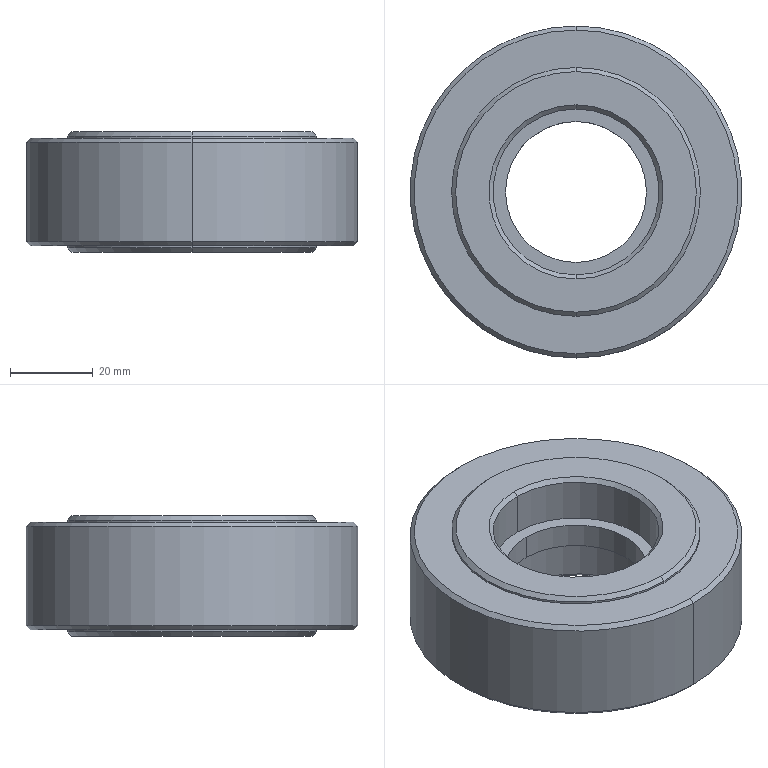Part | SolidWorks | features Chamfer 2, Revolution 2 | 2 solids | 54 faces | box 80 x 80 x 29 mm | volume 104259 mm3 | cylinder 28 | plane 14 | cone 12 | commonest cylinder face diameters 60 x12 54 x8 40 x4 34 x2 80 x2
STEP:
#1=CARTESIAN_POINT('',(0.,39.,-13.));
#2=VERTEX_POINT('',#1);
#3=CARTESIAN_POINT('',(0.,-39.,-13.));
#4=VERTEX_POINT('',#3);
#5=CARTESIAN_POINT('',(0.,0.,-13.));
#6=DIRECTION('',(0.,0.,-1.));
#7=DIRECTION('',(0.,-1.,0.));
#8=AXIS2_PLACEMENT_3D('',#5,#6,#7);
#9=CIRCLE('',#8,39.);
#10=EDGE_CURVE('',#2,#4,#9,.T.);
#11=ORIENTED_EDGE('',*,*,#10,.F.);
#12=CARTESIAN_POINT('',(0.,40.,-12.));
#13=VERTEX_POINT('',#12);
#14=CARTESIAN_POINT('',(0.,40.,-12.));
#15=DIRECTION('',(0.,0.7071,0.7071));
#16=VECTOR('',#15,1000.);
#17=LINE('',#14,#16);
#18=EDGE_CURVE('',#2,#13,#17,.T.);
#19=ORIENTED_EDGE('',*,*,#18,.T.);
#20=CARTESIAN_POINT('',(0.,-40.,-12.));
#21=VERTEX_POINT('',#20);
#22=CARTESIAN_POINT('',(0.,0.,-12.));
#23=DIRECTION('',(0.,0.,1.));
#24=DIRECTION('',(0.,-1.,0.));
#25=AXIS2_PLACEMENT_3D('',#22,#23,#24);
#26=CIRCLE('',#25,40.);
#27=EDGE_CURVE('',#21,#13,#26,.T.);
#28=ORIENTED_EDGE('',*,*,#27,.F.);
#29=CARTESIAN_POINT('',(0.,-40.,-12.));
#30=DIRECTION('',(0.,-0.7071,0.7071));
#31=VECTOR('',#30,1000.);
#32=LINE('',#29,#31);
#33=EDGE_CURVE('',#4,#21,#32,.T.);
#34=ORIENTED_EDGE('',*,*,#33,.F.);
#35=EDGE_LOOP('',(#11,#19,#28,#34));
#36=FACE_OUTER_BOUND('',#35,.T.);
#37=CARTESIAN_POINT('',(0.,0.,-12.));
#38=DIRECTION('',(0.,0.,1.));
#39=DIRECTION('',(0.,-1.,0.));
#40=AXIS2_PLACEMENT_3D('',#37,#38,#39);
#41=CONICAL_SURFACE('',#40,40.,0.7854);
#42=ADVANCED_FACE('',(#36),#41,.T.);
#43=CARTESIAN_POINT('',(0.,-39.,13.));
#44=VERTEX_POINT('',#43);
#45=CARTESIAN_POINT('',(0.,39.,13.));
#46=VERTEX_POINT('',#45);
#47=CARTESIAN_POINT('',(0.,0.,13.));
#48=DIRECTION('',(0.,0.,1.));
#49=DIRECTION('',(0.,-1.,0.));
#50=AXIS2_PLACEMENT_3D('',#47,#48,#49);
#51=CIRCLE('',#50,39.);
#52=EDGE_CURVE('',#44,#46,#51,.T.);
#53=ORIENTED_EDGE('',*,*,#52,.F.);
#54=CARTESIAN_POINT('',(0.,-40.,12.));
#55=VERTEX_POINT('',#54);
#56=CARTESIAN_POINT('',(0.,-39.,13.));
#57=DIRECTION('',(0.,-0.7071,-0.7071));
#58=VECTOR('',#57,1000.);
#59=LINE('',#56,#58);
#60=EDGE_CURVE('',#44,#55,#59,.T.);
#61=ORIENTED_EDGE('',*,*,#60,.T.);
#62=CARTESIAN_POINT('',(0.,40.,12.));
#63=VERTEX_POINT('',#62);
#64=CARTESIAN_POINT('',(0.,0.,12.));
#65=DIRECTION('',(0.,0.,-1.));
#66=DIRECTION('',(0.,-1.,0.));
#67=AXIS2_PLACEMENT_3D('',#64,#65,#66);
#68=CIRCLE('',#67,40.);
#69=EDGE_CURVE('',#63,#55,#68,.T.);
#70=ORIENTED_EDGE('',*,*,#69,.F.);
#71=CARTESIAN_POINT('',(0.,39.,13.));
#72=DIRECTION('',(0.,0.7071,-0.7071));
#73=VECTOR('',#72,1000.);
#74=LINE('',#71,#73);
#75=EDGE_CURVE('',#46,#63,#74,.T.);
#76=ORIENTED_EDGE('',*,*,#75,.F.);
#77=EDGE_LOOP('',(#53,#61,#70,#76));
#78=FACE_OUTER_BOUND('',#77,.T.);
#79=CARTESIAN_POINT('',(0.,0.,13.));
#80=DIRECTION('',(0.,0.,-1.));
#81=DIRECTION('',(0.,1.,0.));
#82=AXIS2_PLACEMENT_3D('',#79,#80,#81);
#83=CONICAL_SURFACE('',#82,39.,0.7854);
#84=ADVANCED_FACE('',(#78),#83,.T.);
#85=CARTESIAN_POINT('',(0.,30.,-3.5));
#86=VERTEX_POINT('',#85);
#87=CARTESIAN_POINT('',(0.,-30.,-3.5));
#88=VERTEX_POINT('',#87);
#89=CARTESIAN_POINT('',(0.,0.,-3.5));
#90=DIRECTION('',(0.,0.,1.));
#91=DIRECTION('',(0.,-1.,0.));
#92=AXIS2_PLACEMENT_3D('',#89,#90,#91);
#93=CIRCLE('',#92,30.);
#94=EDGE_CURVE('',#86,#88,#93,.T.);
#95=ORIENTED_EDGE('',*,*,#94,.F.);
#96=CARTESIAN_POINT('',(0.,30.,3.5));
#97=VERTEX_POINT('',#96);
#98=CARTESIAN_POINT('',(0.,30.,13.));
#99=DIRECTION('',(0.,0.,1.));
#100=VECTOR('',#99,1000.);
#101=LINE('',#98,#100);
#102=EDGE_CURVE('',#86,#97,#101,.T.);
#103=ORIENTED_EDGE('',*,*,#102,.T.);
#104=CARTESIAN_POINT('',(0.,-30.,3.5));
#105=VERTEX_POINT('',#104);
#106=CARTESIAN_POINT('',(0.,0.,3.5));
#107=DIRECTION('',(0.,0.,1.));
#108=DIRECTION('',(0.,-1.,0.));
#109=AXIS2_PLACEMENT_3D('',#106,#107,#108);
#110=CIRCLE('',#109,30.);
#111=EDGE_CURVE('',#97,#105,#110,.T.);
#112=ORIENTED_EDGE('',*,*,#111,.T.);
#113=CARTESIAN_POINT('',(0.,-30.,13.));
#114=DIRECTION('',(0.,0.,1.));
#115=VECTOR('',#114,1000.);
#116=LINE('',#113,#115);
#117=EDGE_CURVE('',#88,#105,#116,.T.);
#118=ORIENTED_EDGE('',*,*,#117,.F.);
#119=EDGE_LOOP('',(#95,#103,#112,#118));
#120=FACE_OUTER_BOUND('',#119,.T.);
#121=CARTESIAN_POINT('',(0.,0.,13.));
#122=DIRECTION('',(0.,0.,1.));
#123=DIRECTION('',(0.,-1.,0.));
#124=AXIS2_PLACEMENT_3D('',#121,#122,#123);
#125=CYLINDRICAL_SURFACE('',#124,30.);
#126=ADVANCED_FACE('',(#120),#125,.F.);
#127=CARTESIAN_POINT('',(0.,27.,3.5));
#128=VERTEX_POINT('',#127);
#129=CARTESIAN_POINT('',(0.,-27.,3.5));
#130=VERTEX_POINT('',#129);
#131=CARTESIAN_POINT('',(0.,0.,3.5));
#132=DIRECTION('',(0.,0.,1.));
#133=DIRECTION('',(0.,-1.,0.));
#134=AXIS2_PLACEMENT_3D('',#131,#132,#133);
#135=CIRCLE('',#134,27.);
#136=EDGE_CURVE('',#128,#130,#135,.T.);
#137=ORIENTED_EDGE('',*,*,#136,.F.);
#138=CARTESIAN_POINT('',(0.,27.,9.5));
#139=VERTEX_POINT('',#138);
#140=CARTESIAN_POINT('',(0.,27.,13.));
#141=DIRECTION('',(0.,0.,1.));
#142=VECTOR('',#141,1000.);
#143=LINE('',#140,#142);
#144=EDGE_CURVE('',#128,#139,#143,.T.);
#145=ORIENTED_EDGE('',*,*,#144,.T.);
#146=CARTESIAN_POINT('',(0.,-27.,9.5));
#147=VERTEX_POINT('',#146);
#148=CARTESIAN_POINT('',(0.,0.,9.5));
#149=DIRECTION('',(0.,0.,1.));
#150=DIRECTION('',(0.,-1.,0.));
#151=AXIS2_PLACEMENT_3D('',#148,#149,#150);
#152=CIRCLE('',#151,27.);
#153=EDGE_CURVE('',#139,#147,#152,.T.);
#154=ORIENTED_EDGE('',*,*,#153,.T.);
#155=CARTESIAN_POINT('',(0.,-27.,13.));
#156=DIRECTION('',(0.,0.,1.));
#157=VECTOR('',#156,1000.);
#158=LINE('',#155,#157);
#159=EDGE_CURVE('',#130,#147,#158,.T.);
#160=ORIENTED_EDGE('',*,*,#159,.F.);
#161=EDGE_LOOP('',(#137,#145,#154,#160));
#162=FACE_OUTER_BOUND('',#161,.T.);
#163=CARTESIAN_POINT('',(0.,0.,13.));
#164=DIRECTION('',(0.,0.,1.));
#165=DIRECTION('',(0.,-1.,0.));
#166=AXIS2_PLACEMENT_3D('',#163,#164,#165);
#167=CYLINDRICAL_SURFACE('',#166,27.);
#168=ADVANCED_FACE('',(#162),#167,.F.);
#169=CARTESIAN_POINT('',(0.,30.,9.5));
#170=VERTEX_POINT('',#169);
#171=CARTESIAN_POINT('',(0.,-30.,9.5));
#172=VERTEX_POINT('',#171);
#173=CARTESIAN_POINT('',(0.,0.,9.5));
#174=DIRECTION('',(0.,0.,1.));
#175=DIRECTION('',(0.,-1.,0.));
#176=AXIS2_PLACEMENT_3D('',#173,#174,#175);
#177=CIRCLE('',#176,30.);
#178=EDGE_CURVE('',#170,#172,#177,.T.);
#179=ORIENTED_EDGE('',*,*,#178,.F.);
#180=CARTESIAN_POINT('',(0.,30.,13.));
#181=VERTEX_POINT('',#180);
#182=CARTESIAN_POINT('',(0.,30.,13.));
#183=DIRECTION('',(0.,0.,1.));
#184=VECTOR('',#183,1000.);
#185=LINE('',#182,#184);
#186=EDGE_CURVE('',#170,#181,#185,.T.);
#187=ORIENTED_EDGE('',*,*,#186,.T.);
#188=CARTESIAN_POINT('',(0.,-30.,13.));
#189=VERTEX_POINT('',#188);
#190=CARTESIAN_POINT('',(0.,0.,13.));
#191=DIRECTION('',(0.,0.,1.));
#192=DIRECTION('',(0.,-1.,0.));
#193=AXIS2_PLACEMENT_3D('',#190,#191,#192);
#194=CIRCLE('',#193,30.);
#195=EDGE_CURVE('',#181,#189,#194,.T.);
#196=ORIENTED_EDGE('',*,*,#195,.T.);
#197=CARTESIAN_POINT('',(0.,-30.,13.));
#198=DIRECTION('',(0.,0.,1.));
#199=VECTOR('',#198,1000.);
#200=LINE('',#197,#199);
#201=EDGE_CURVE('',#172,#189,#200,.T.);
#202=ORIENTED_EDGE('',*,*,#201,.F.);
#203=EDGE_LOOP('',(#179,#187,#196,#202));
#204=FACE_OUTER_BOUND('',#203,.T.);
#205=CARTESIAN_POINT('',(0.,0.,13.));
#206=DIRECTION('',(0.,0.,1.));
#207=DIRECTION('',(0.,-1.,0.));
#208=AXIS2_PLACEMENT_3D('',#205,#206,#207);
#209=CYLINDRICAL_SURFACE('',#208,30.);
#210=ADVANCED_FACE('',(#204),#209,.F.);
#211=ORIENTED_EDGE('',*,*,#27,.T.);
#212=CARTESIAN_POINT('',(0.,40.,13.));
#213=DIRECTION('',(0.,0.,1.));
#214=VECTOR('',#213,1000.);
#215=LINE('',#212,#214);
#216=EDGE_CURVE('',#13,#63,#215,.T.);
#217=ORIENTED_EDGE('',*,*,#216,.T.);
#218=ORIENTED_EDGE('',*,*,#69,.T.);
#219=CARTESIAN_POINT('',(0.,-40.,13.));
#220=DIRECTION('',(0.,0.,1.));
#221=VECTOR('',#220,1000.);
#222=LINE('',#219,#221);
#223=EDGE_CURVE('',#21,#55,#222,.T.);
#224=ORIENTED_EDGE('',*,*,#223,.F.);
#225=EDGE_LOOP('',(#211,#217,#218,#224));
#226=FACE_OUTER_BOUND('',#225,.T.);
#227=CARTESIAN_POINT('',(0.,0.,13.));
#228=DIRECTION('',(0.,0.,1.));
#229=DIRECTION('',(0.,-1.,0.));
#230=AXIS2_PLACEMENT_3D('',#227,#228,#229);
#231=CYLINDRICAL_SURFACE('',#230,40.);
#232=ADVANCED_FACE('',(#226),#231,.T.);
#233=CARTESIAN_POINT('',(0.,30.,-13.));
#234=VERTEX_POINT('',#233);
#235=CARTESIAN_POINT('',(0.,-30.,-13.));
#236=VERTEX_POINT('',#235);
#237=CARTESIAN_POINT('',(0.,0.,-13.));
#238=DIRECTION('',(0.,0.,1.));
#239=DIRECTION('',(0.,-1.,0.));
#240=AXIS2_PLACEMENT_3D('',#237,#238,#239);
#241=CIRCLE('',#240,30.);
#242=EDGE_CURVE('',#234,#236,#241,.T.);
#243=ORIENTED_EDGE('',*,*,#242,.F.);
#244=CARTESIAN_POINT('',(0.,30.,-9.5));
#245=VERTEX_POINT('',#244);
#246=CARTESIAN_POINT('',(0.,30.,13.));
#247=DIRECTION('',(0.,0.,1.));
#248=VECTOR('',#247,1000.);
#249=LINE('',#246,#248);
#250=EDGE_CURVE('',#234,#245,#249,.T.);
#251=ORIENTED_EDGE('',*,*,#250,.T.);
#252=CARTESIAN_POINT('',(0.,-30.,-9.5));
#253=VERTEX_POINT('',#252);
#254=CARTESIAN_POINT('',(0.,0.,-9.5));
#255=DIRECTION('',(0.,0.,1.));
#256=DIRECTION('',(0.,-1.,0.));
#257=AXIS2_PLACEMENT_3D('',#254,#255,#256);
#258=CIRCLE('',#257,30.);
#259=EDGE_CURVE('',#245,#253,#258,.T.);
#260=ORIENTED_EDGE('',*,*,#259,.T.);
#261=CARTESIAN_POINT('',(0.,-30.,13.));
#262=DIRECTION('',(0.,0.,1.));
#263=VECTOR('',#262,1000.);
#264=LINE('',#261,#263);
#265=EDGE_CURVE('',#236,#253,#264,.T.);
#266=ORIENTED_EDGE('',*,*,#265,.F.);
#267=EDGE_LOOP('',(#243,#251,#260,#266));
#268=FACE_OUTER_BOUND('',#267,.T.);
#269=CARTESIAN_POINT('',(0.,0.,13.));
#270=DIRECTION('',(0.,0.,1.));
#271=DIRECTION('',(0.,-1.,0.));
#272=AXIS2_PLACEMENT_3D('',#269,#270,#271);
#273=CYLINDRICAL_SURFACE('',#272,30.);
#274=ADVANCED_FACE('',(#268),#273,.F.);
#275=CARTESIAN_POINT('',(0.,27.,-9.5));
#276=VERTEX_POINT('',#275);
#277=CARTESIAN_POINT('',(0.,-27.,-9.5));
#278=VERTEX_POINT('',#277);
#279=CARTESIAN_POINT('',(0.,0.,-9.5));
#280=DIRECTION('',(0.,0.,1.));
#281=DIRECTION('',(0.,-1.,0.));
#282=AXIS2_PLACEMENT_3D('',#279,#280,#281);
#283=CIRCLE('',#282,27.);
#284=EDGE_CURVE('',#276,#278,#283,.T.);
#285=ORIENTED_EDGE('',*,*,#284,.F.);
#286=CARTESIAN_POINT('',(0.,27.,-3.5));
#287=VERTEX_POINT('',#286);
#288=CARTESIAN_POINT('',(0.,27.,13.));
#289=DIRECTION('',(0.,0.,1.));
#290=VECTOR('',#289,1000.);
#291=LINE('',#288,#290);
#292=EDGE_CURVE('',#276,#287,#291,.T.);
#293=ORIENTED_EDGE('',*,*,#292,.T.);
#294=CARTESIAN_POINT('',(0.,-27.,-3.5));
#295=VERTEX_POINT('',#294);
#296=CARTESIAN_POINT('',(0.,0.,-3.5));
#297=DIRECTION('',(0.,0.,1.));
#298=DIRECTION('',(0.,-1.,0.));
#299=AXIS2_PLACEMENT_3D('',#296,#297,#298);
#300=CIRCLE('',#299,27.);
#301=EDGE_CURVE('',#287,#295,#300,.T.);
#302=ORIENTED_EDGE('',*,*,#301,.T.);
#303=CARTESIAN_POINT('',(0.,-27.,13.));
#304=DIRECTION('',(0.,0.,1.));
#305=VECTOR('',#304,1000.);
#306=LINE('',#303,#305);
#307=EDGE_CURVE('',#278,#295,#306,.T.);
#308=ORIENTED_EDGE('',*,*,#307,.F.);
#309=EDGE_LOOP('',(#285,#293,#302,#308));
#310=FACE_OUTER_BOUND('',#309,.T.);
#311=CARTESIAN_POINT('',(0.,0.,13.));
#312=DIRECTION('',(0.,0.,1.));
#313=DIRECTION('',(0.,-1.,0.));
#314=AXIS2_PLACEMENT_3D('',#311,#312,#313);
#315=CYLINDRICAL_SURFACE('',#314,27.);
#316=ADVANCED_FACE('',(#310),#315,.F.);
#317=ORIENTED_EDGE('',*,*,#292,.F.);
#318=CARTESIAN_POINT('',(0.,0.,-9.5));
#319=DIRECTION('',(0.,0.,1.));
#320=DIRECTION('',(0.,-1.,0.));
#321=AXIS2_PLACEMENT_3D('',#318,#319,#320);
#322=CIRCLE('',#321,27.);
#323=EDGE_CURVE('',#278,#276,#322,.T.);
#324=ORIENTED_EDGE('',*,*,#323,.F.);
#325=ORIENTED_EDGE('',*,*,#307,.T.);
#326=CARTESIAN_POINT('',(0.,0.,-3.5));
#327=DIRECTION('',(0.,0.,1.));
#328=DIRECTION('',(0.,-1.,0.));
#329=AXIS2_PLACEMENT_3D('',#326,#327,#328);
#330=CIRCLE('',#329,27.);
#331=EDGE_CURVE('',#295,#287,#330,.T.);
#332=ORIENTED_EDGE('',*,*,#331,.T.);
#333=EDGE_LOOP('',(#317,#324,#325,#332));
#334=FACE_OUTER_BOUND('',#333,.T.);
#335=CARTESIAN_POINT('',(0.,0.,13.));
#336=DIRECTION('',(0.,0.,1.));
#337=DIRECTION('',(0.,-1.,0.));
#338=AXIS2_PLACEMENT_3D('',#335,#336,#337);
#339=CYLINDRICAL_SURFACE('',#338,27.);
#340=ADVANCED_FACE('',(#334),#339,.F.);
#341=ORIENTED_EDGE('',*,*,#323,.T.);
#342=ORIENTED_EDGE('',*,*,#284,.T.);
#343=EDGE_LOOP('',(#341,#342));
#344=FACE_BOUND('',#343,.T.);
#345=CARTESIAN_POINT('',(0.,0.,-9.5));
#346=DIRECTION('',(0.,0.,1.));
#347=DIRECTION('',(0.,-1.,0.));
#348=AXIS2_PLACEMENT_3D('',#345,#346,#347);
#349=CIRCLE('',#348,30.);
#350=EDGE_CURVE('',#253,#245,#349,.T.);
#351=ORIENTED_EDGE('',*,*,#350,.F.);
#352=ORIENTED_EDGE('',*,*,#259,.F.);
#353=EDGE_LOOP('',(#351,#352));
#354=FACE_OUTER_BOUND('',#353,.T.);
#355=CARTESIAN_POINT('',(0.,0.,-9.5));
#356=DIRECTION('',(0.,0.,-1.));
#357=DIRECTION('',(0.,1.,0.));
#358=AXIS2_PLACEMENT_3D('',#355,#356,#357);
#359=PLANE('',#358);
#360=ADVANCED_FACE('',(#344,#354),#359,.T.);
#361=ORIENTED_EDGE('',*,*,#250,.F.);
#362=CARTESIAN_POINT('',(0.,0.,-13.));
#363=DIRECTION('',(0.,0.,1.));
#364=DIRECTION('',(0.,-1.,0.));
#365=AXIS2_PLACEMENT_3D('',#362,#363,#364);
#366=CIRCLE('',#365,30.);
#367=EDGE_CURVE('',#236,#234,#366,.T.);
#368=ORIENTED_EDGE('',*,*,#367,.F.);
#369=ORIENTED_EDGE('',*,*,#265,.T.);
#370=ORIENTED_EDGE('',*,*,#350,.T.);
#371=EDGE_LOOP('',(#361,#368,#369,#370));
#372=FACE_OUTER_BOUND('',#371,.T.);
#373=CARTESIAN_POINT('',(0.,0.,13.));
#374=DIRECTION('',(0.,0.,1.));
#375=DIRECTION('',(0.,-1.,0.));
#376=AXIS2_PLACEMENT_3D('',#373,#374,#375);
#377=CYLINDRICAL_SURFACE('',#376,30.);
#378=ADVANCED_FACE('',(#372),#377,.F.);
#379=CARTESIAN_POINT('',(0.,0.,-13.));
#380=DIRECTION('',(0.,0.,-1.));
#381=DIRECTION('',(0.,-1.,0.));
#382=AXIS2_PLACEMENT_3D('',#379,#380,#381);
#383=CIRCLE('',#382,39.);
#384=EDGE_CURVE('',#4,#2,#383,.T.);
#385=ORIENTED_EDGE('',*,*,#384,.T.);
#386=ORIENTED_EDGE('',*,*,#10,.T.);
#387=EDGE_LOOP('',(#385,#386));
#388=FACE_OUTER_BOUND('',#387,.T.);
#389=ORIENTED_EDGE('',*,*,#367,.T.);
#390=ORIENTED_EDGE('',*,*,#242,.T.);
#391=EDGE_LOOP('',(#389,#390));
#392=FACE_BOUND('',#391,.T.);
#393=CARTESIAN_POINT('',(0.,0.,-13.));
#394=DIRECTION('',(0.,0.,1.));
#395=DIRECTION('',(0.,-1.,0.));
#396=AXIS2_PLACEMENT_3D('',#393,#394,#395);
#397=PLANE('',#396);
#398=ADVANCED_FACE('',(#388,#392),#397,.F.);
#399=ORIENTED_EDGE('',*,*,#216,.F.);
#400=CARTESIAN_POINT('',(0.,0.,-12.));
#401=DIRECTION('',(0.,0.,1.));
#402=DIRECTION('',(0.,-1.,0.));
#403=AXIS2_PLACEMENT_3D('',#400,#401,#402);
#404=CIRCLE('',#403,40.);
#405=EDGE_CURVE('',#13,#21,#404,.T.);
#406=ORIENTED_EDGE('',*,*,#405,.T.);
#407=ORIENTED_EDGE('',*,*,#223,.T.);
#408=CARTESIAN_POINT('',(0.,0.,12.));
#409=DIRECTION('',(0.,0.,-1.));
#410=DIRECTION('',(0.,-1.,0.));
#411=AXIS2_PLACEMENT_3D('',#408,#409,#410);
#412=CIRCLE('',#411,40.);
#413=EDGE_CURVE('',#55,#63,#412,.T.);
#414=ORIENTED_EDGE('',*,*,#413,.T.);
#415=EDGE_LOOP('',(#399,#406,#407,#414));
#416=FACE_OUTER_BOUND('',#415,.T.);
#417=CARTESIAN_POINT('',(0.,0.,13.));
#418=DIRECTION('',(0.,0.,1.));
#419=DIRECTION('',(0.,-1.,0.));
#420=AXIS2_PLACEMENT_3D('',#417,#418,#419);
#421=CYLINDRICAL_SURFACE('',#420,40.);
#422=ADVANCED_FACE('',(#416),#421,.T.);
#423=CARTESIAN_POINT('',(0.,0.,13.));
#424=DIRECTION('',(0.,0.,1.));
#425=DIRECTION('',(0.,-1.,0.));
#426=AXIS2_PLACEMENT_3D('',#423,#424,#425);
#427=CIRCLE('',#426,39.);
#428=EDGE_CURVE('',#46,#44,#427,.T.);
#429=ORIENTED_EDGE('',*,*,#428,.T.);
#430=ORIENTED_EDGE('',*,*,#52,.T.);
#431=EDGE_LOOP('',(#429,#430));
#432=FACE_OUTER_BOUND('',#431,.T.);
#433=CARTESIAN_POINT('',(0.,0.,13.));
#434=DIRECTION('',(0.,0.,1.));
#435=DIRECTION('',(0.,-1.,0.));
#436=AXIS2_PLACEMENT_3D('',#433,#434,#435);
#437=CIRCLE('',#436,30.);
#438=EDGE_CURVE('',#189,#181,#437,.T.);
#439=ORIENTED_EDGE('',*,*,#438,.F.);
#440=ORIENTED_EDGE('',*,*,#195,.F.);
#441=EDGE_LOOP('',(#439,#440));
#442=FACE_BOUND('',#441,.T.);
#443=CARTESIAN_POINT('',(0.,0.,13.));
#444=DIRECTION('',(0.,0.,1.));
#445=DIRECTION('',(0.,-1.,0.));
#446=AXIS2_PLACEMENT_3D('',#443,#444,#445);
#447=PLANE('',#446);
#448=ADVANCED_FACE('',(#432,#442),#447,.T.);
#449=ORIENTED_EDGE('',*,*,#186,.F.);
#450=CARTESIAN_POINT('',(0.,0.,9.5));
#451=DIRECTION('',(0.,0.,1.));
#452=DIRECTION('',(0.,-1.,0.));
#453=AXIS2_PLACEMENT_3D('',#450,#451,#452);
#454=CIRCLE('',#453,30.);
#455=EDGE_CURVE('',#172,#170,#454,.T.);
#456=ORIENTED_EDGE('',*,*,#455,.F.);
#457=ORIENTED_EDGE('',*,*,#201,.T.);
#458=ORIENTED_EDGE('',*,*,#438,.T.);
#459=EDGE_LOOP('',(#449,#456,#457,#458));
#460=FACE_OUTER_BOUND('',#459,.T.);
#461=CARTESIAN_POINT('',(0.,0.,13.));
#462=DIRECTION('',(0.,0.,1.));
#463=DIRECTION('',(0.,-1.,0.));
#464=AXIS2_PLACEMENT_3D('',#461,#462,#463);
#465=CYLINDRICAL_SURFACE('',#464,30.);
#466=ADVANCED_FACE('',(#460),#465,.F.);
#467=CARTESIAN_POINT('',(0.,0.,9.5));
#468=DIRECTION('',(0.,0.,1.));
#469=DIRECTION('',(0.,-1.,0.));
#470=AXIS2_PLACEMENT_3D('',#467,#468,#469);
#471=CIRCLE('',#470,27.);
#472=EDGE_CURVE('',#147,#139,#471,.T.);
#473=ORIENTED_EDGE('',*,*,#472,.F.);
#474=ORIENTED_EDGE('',*,*,#153,.F.);
#475=EDGE_LOOP('',(#473,#474));
#476=FACE_BOUND('',#475,.T.);
#477=ORIENTED_EDGE('',*,*,#455,.T.);
#478=ORIENTED_EDGE('',*,*,#178,.T.);
#479=EDGE_LOOP('',(#477,#478));
#480=FACE_OUTER_BOUND('',#479,.T.);
#481=CARTESIAN_POINT('',(0.,0.,9.5));
#482=DIRECTION('',(0.,0.,-1.));
#483=DIRECTION('',(0.,1.,0.));
#484=AXIS2_PLACEMENT_3D('',#481,#482,#483);
#485=PLANE('',#484);
#486=ADVANCED_FACE('',(#476,#480),#485,.F.);
#487=ORIENTED_EDGE('',*,*,#144,.F.);
#488=CARTESIAN_POINT('',(0.,0.,3.5));
#489=DIRECTION('',(0.,0.,1.));
#490=DIRECTION('',(0.,-1.,0.));
#491=AXIS2_PLACEMENT_3D('',#488,#489,#490);
#492=CIRCLE('',#491,27.);
#493=EDGE_CURVE('',#130,#128,#492,.T.);
#494=ORIENTED_EDGE('',*,*,#493,.F.);
#495=ORIENTED_EDGE('',*,*,#159,.T.);
#496=ORIENTED_EDGE('',*,*,#472,.T.);
#497=EDGE_LOOP('',(#487,#494,#495,#496));
#498=FACE_OUTER_BOUND('',#497,.T.);
#499=CARTESIAN_POINT('',(0.,0.,13.));
#500=DIRECTION('',(0.,0.,1.));
#501=DIRECTION('',(0.,-1.,0.));
#502=AXIS2_PLACEMENT_3D('',#499,#500,#501);
#503=CYLINDRICAL_SURFACE('',#502,27.);
#504=ADVANCED_FACE('',(#498),#503,.F.);
#505=CARTESIAN_POINT('',(0.,0.,3.5));
#506=DIRECTION('',(0.,0.,1.));
#507=DIRECTION('',(0.,-1.,0.));
#508=AXIS2_PLACEMENT_3D('',#505,#506,#507);
#509=CIRCLE('',#508,30.);
#510=EDGE_CURVE('',#105,#97,#509,.T.);
#511=ORIENTED_EDGE('',*,*,#510,.F.);
#512=ORIENTED_EDGE('',*,*,#111,.F.);
#513=EDGE_LOOP('',(#511,#512));
#514=FACE_OUTER_BOUND('',#513,.T.);
#515=ORIENTED_EDGE('',*,*,#493,.T.);
#516=ORIENTED_EDGE('',*,*,#136,.T.);
#517=EDGE_LOOP('',(#515,#516));
#518=FACE_BOUND('',#517,.T.);
#519=CARTESIAN_POINT('',(0.,0.,3.5));
#520=DIRECTION('',(0.,0.,1.));
#521=DIRECTION('',(0.,-1.,0.));
#522=AXIS2_PLACEMENT_3D('',#519,#520,#521);
#523=PLANE('',#522);
#524=ADVANCED_FACE('',(#514,#518),#523,.F.);
#525=ORIENTED_EDGE('',*,*,#102,.F.);
#526=CARTESIAN_POINT('',(0.,0.,-3.5));
#527=DIRECTION('',(0.,0.,1.));
#528=DIRECTION('',(0.,-1.,0.));
#529=AXIS2_PLACEMENT_3D('',#526,#527,#528);
#530=CIRCLE('',#529,30.);
#531=EDGE_CURVE('',#88,#86,#530,.T.);
#532=ORIENTED_EDGE('',*,*,#531,.F.);
#533=ORIENTED_EDGE('',*,*,#117,.T.);
#534=ORIENTED_EDGE('',*,*,#510,.T.);
#535=EDGE_LOOP('',(#525,#532,#533,#534));
#536=FACE_OUTER_BOUND('',#535,.T.);
#537=CARTESIAN_POINT('',(0.,0.,13.));
#538=DIRECTION('',(0.,0.,1.));
#539=DIRECTION('',(0.,-1.,0.));
#540=AXIS2_PLACEMENT_3D('',#537,#538,#539);
#541=CYLINDRICAL_SURFACE('',#540,30.);
#542=ADVANCED_FACE('',(#536),#541,.F.);
#543=ORIENTED_EDGE('',*,*,#531,.T.);
#544=ORIENTED_EDGE('',*,*,#94,.T.);
#545=EDGE_LOOP('',(#543,#544));
#546=FACE_OUTER_BOUND('',#545,.T.);
#547=ORIENTED_EDGE('',*,*,#331,.F.);
#548=ORIENTED_EDGE('',*,*,#301,.F.);
#549=EDGE_LOOP('',(#547,#548));
#550=FACE_BOUND('',#549,.T.);
#551=CARTESIAN_POINT('',(0.,0.,-3.5));
#552=DIRECTION('',(0.,0.,1.));
#553=DIRECTION('',(0.,-1.,0.));
#554=AXIS2_PLACEMENT_3D('',#551,#552,#553);
#555=PLANE('',#554);
#556=ADVANCED_FACE('',(#546,#550),#555,.T.);
#557=ORIENTED_EDGE('',*,*,#60,.F.);
#558=ORIENTED_EDGE('',*,*,#428,.F.);
#559=ORIENTED_EDGE('',*,*,#75,.T.);
#560=ORIENTED_EDGE('',*,*,#413,.F.);
#561=EDGE_LOOP('',(#557,#558,#559,#560));
#562=FACE_OUTER_BOUND('',#561,.T.);
#563=CARTESIAN_POINT('',(0.,0.,13.));
#564=DIRECTION('',(0.,0.,-1.));
#565=DIRECTION('',(0.,1.,0.));
#566=AXIS2_PLACEMENT_3D('',#563,#564,#565);
#567=CONICAL_SURFACE('',#566,39.,0.7854);
#568=ADVANCED_FACE('',(#562),#567,.T.);
#569=ORIENTED_EDGE('',*,*,#18,.F.);
#570=ORIENTED_EDGE('',*,*,#384,.F.);
#571=ORIENTED_EDGE('',*,*,#33,.T.);
#572=ORIENTED_EDGE('',*,*,#405,.F.);
#573=EDGE_LOOP('',(#569,#570,#571,#572));
#574=FACE_OUTER_BOUND('',#573,.T.);
#575=CARTESIAN_POINT('',(0.,0.,-12.));
#576=DIRECTION('',(0.,0.,1.));
#577=DIRECTION('',(0.,-1.,0.));
#578=AXIS2_PLACEMENT_3D('',#575,#576,#577);
#579=CONICAL_SURFACE('',#578,40.,0.7854);
#580=ADVANCED_FACE('',(#574),#579,.T.);
#581=CLOSED_SHELL('',(#42,#84,#126,#168,#210,#232,#274,#316,#340,#360,#378,#398,#422,#448,#466,#486,#504,#524,#542,#556,#568,#580));
#582=MANIFOLD_SOLID_BREP('',#581);
#583=CARTESIAN_POINT('',(0.,-29.,14.5));
#584=VERTEX_POINT('',#583);
#585=CARTESIAN_POINT('',(0.,29.,14.5));
#586=VERTEX_POINT('',#585);
#587=CARTESIAN_POINT('',(0.,0.,14.5));
#588=DIRECTION('',(0.,0.,1.));
#589=DIRECTION('',(0.,-1.,0.));
#590=AXIS2_PLACEMENT_3D('',#587,#588,#589);
#591=CIRCLE('',#590,29.);
#592=EDGE_CURVE('',#584,#586,#591,.T.);
#593=ORIENTED_EDGE('',*,*,#592,.F.);
#594=CARTESIAN_POINT('',(0.,-30.,13.5));
#595=VERTEX_POINT('',#594);
#596=CARTESIAN_POINT('',(0.,-29.,14.5));
#597=DIRECTION('',(0.,-0.7071,-0.7071));
#598=VECTOR('',#597,1000.);
#599=LINE('',#596,#598);
#600=EDGE_CURVE('',#584,#595,#599,.T.);
#601=ORIENTED_EDGE('',*,*,#600,.T.);
#602=CARTESIAN_POINT('',(0.,30.,13.5));
#603=VERTEX_POINT('',#602);
#604=CARTESIAN_POINT('',(0.,0.,13.5));
#605=DIRECTION('',(0.,0.,-1.));
#606=DIRECTION('',(0.,-1.,0.));
#607=AXIS2_PLACEMENT_3D('',#604,#605,#606);
#608=CIRCLE('',#607,30.);
#609=EDGE_CURVE('',#603,#595,#608,.T.);
#610=ORIENTED_EDGE('',*,*,#609,.F.);
#611=CARTESIAN_POINT('',(0.,29.,14.5));
#612=DIRECTION('',(0.,0.7071,-0.7071));
#613=VECTOR('',#612,1000.);
#614=LINE('',#611,#613);
#615=EDGE_CURVE('',#586,#603,#614,.T.);
#616=ORIENTED_EDGE('',*,*,#615,.F.);
#617=EDGE_LOOP('',(#593,#601,#610,#616));
#618=FACE_OUTER_BOUND('',#617,.T.);
#619=CARTESIAN_POINT('',(0.,0.,14.5));
#620=DIRECTION('',(0.,0.,-1.));
#621=DIRECTION('',(0.,1.,0.));
#622=AXIS2_PLACEMENT_3D('',#619,#620,#621);
#623=CONICAL_SURFACE('',#622,29.,0.7854);
#624=ADVANCED_FACE('',(#618),#623,.T.);
#625=CARTESIAN_POINT('',(0.,20.,13.5));
#626=VERTEX_POINT('',#625);
#627=CARTESIAN_POINT('',(0.,-20.,13.5));
#628=VERTEX_POINT('',#627);
#629=CARTESIAN_POINT('',(0.,0.,13.5));
#630=DIRECTION('',(0.,0.,1.));
#631=DIRECTION('',(0.,-1.,0.));
#632=AXIS2_PLACEMENT_3D('',#629,#630,#631);
#633=CIRCLE('',#632,20.);
#634=EDGE_CURVE('',#626,#628,#633,.T.);
#635=ORIENTED_EDGE('',*,*,#634,.F.);
#636=CARTESIAN_POINT('',(0.,21.,14.5));
#637=VERTEX_POINT('',#636);
#638=CARTESIAN_POINT('',(0.,20.,13.5));
#639=DIRECTION('',(0.,0.7071,0.7071));
#640=VECTOR('',#639,1000.);
#641=LINE('',#638,#640);
#642=EDGE_CURVE('',#626,#637,#641,.T.);
#643=ORIENTED_EDGE('',*,*,#642,.T.);
#644=CARTESIAN_POINT('',(0.,-21.,14.5));
#645=VERTEX_POINT('',#644);
#646=CARTESIAN_POINT('',(0.,0.,14.5));
#647=DIRECTION('',(0.,0.,-1.));
#648=DIRECTION('',(0.,-1.,0.));
#649=AXIS2_PLACEMENT_3D('',#646,#647,#648);
#650=CIRCLE('',#649,21.);
#651=EDGE_CURVE('',#645,#637,#650,.T.);
#652=ORIENTED_EDGE('',*,*,#651,.F.);
#653=CARTESIAN_POINT('',(0.,-20.,13.5));
#654=DIRECTION('',(0.,-0.7071,0.7071));
#655=VECTOR('',#654,1000.);
#656=LINE('',#653,#655);
#657=EDGE_CURVE('',#628,#645,#656,.T.);
#658=ORIENTED_EDGE('',*,*,#657,.F.);
#659=EDGE_LOOP('',(#635,#643,#652,#658));
#660=FACE_OUTER_BOUND('',#659,.T.);
#661=CARTESIAN_POINT('',(0.,0.,13.5));
#662=DIRECTION('',(0.,0.,1.));
#663=DIRECTION('',(0.,-1.,0.));
#664=AXIS2_PLACEMENT_3D('',#661,#662,#663);
#665=CONICAL_SURFACE('',#664,20.,0.7854);
#666=ADVANCED_FACE('',(#660),#665,.F.);
#667=CARTESIAN_POINT('',(0.,29.,-14.5));
#668=VERTEX_POINT('',#667);
#669=CARTESIAN_POINT('',(0.,-29.,-14.5));
#670=VERTEX_POINT('',#669);
#671=CARTESIAN_POINT('',(0.,0.,-14.5));
#672=DIRECTION('',(0.,0.,-1.));
#673=DIRECTION('',(0.,-1.,0.));
#674=AXIS2_PLACEMENT_3D('',#671,#672,#673);
#675=CIRCLE('',#674,29.);
#676=EDGE_CURVE('',#668,#670,#675,.T.);
#677=ORIENTED_EDGE('',*,*,#676,.F.);
#678=CARTESIAN_POINT('',(0.,30.,-13.5));
#679=VERTEX_POINT('',#678);
#680=CARTESIAN_POINT('',(0.,30.,-13.5));
#681=DIRECTION('',(0.,0.7071,0.7071));
#682=VECTOR('',#681,1000.);
#683=LINE('',#680,#682);
#684=EDGE_CURVE('',#668,#679,#683,.T.);
#685=ORIENTED_EDGE('',*,*,#684,.T.);
#686=CARTESIAN_POINT('',(0.,-30.,-13.5));
#687=VERTEX_POINT('',#686);
#688=CARTESIAN_POINT('',(0.,0.,-13.5));
#689=DIRECTION('',(0.,0.,1.));
#690=DIRECTION('',(0.,-1.,0.));
#691=AXIS2_PLACEMENT_3D('',#688,#689,#690);
#692=CIRCLE('',#691,30.);
#693=EDGE_CURVE('',#687,#679,#692,.T.);
#694=ORIENTED_EDGE('',*,*,#693,.F.);
#695=CARTESIAN_POINT('',(0.,-30.,-13.5));
#696=DIRECTION('',(0.,-0.7071,0.7071));
#697=VECTOR('',#696,1000.);
#698=LINE('',#695,#697);
#699=EDGE_CURVE('',#670,#687,#698,.T.);
#700=ORIENTED_EDGE('',*,*,#699,.F.);
#701=EDGE_LOOP('',(#677,#685,#694,#700));
#702=FACE_OUTER_BOUND('',#701,.T.);
#703=CARTESIAN_POINT('',(0.,0.,-13.5));
#704=DIRECTION('',(0.,0.,1.));
#705=DIRECTION('',(0.,-1.,0.));
#706=AXIS2_PLACEMENT_3D('',#703,#704,#705);
#707=CONICAL_SURFACE('',#706,30.,0.7854);
#708=ADVANCED_FACE('',(#702),#707,.T.);
#709=CARTESIAN_POINT('',(0.,-20.,-13.5));
#710=VERTEX_POINT('',#709);
#711=CARTESIAN_POINT('',(0.,20.,-13.5));
#712=VERTEX_POINT('',#711);
#713=CARTESIAN_POINT('',(0.,0.,-13.5));
#714=DIRECTION('',(0.,0.,-1.));
#715=DIRECTION('',(0.,-1.,0.));
#716=AXIS2_PLACEMENT_3D('',#713,#714,#715);
#717=CIRCLE('',#716,20.);
#718=EDGE_CURVE('',#710,#712,#717,.T.);
#719=ORIENTED_EDGE('',*,*,#718,.F.);
#720=CARTESIAN_POINT('',(0.,-21.,-14.5));
#721=VERTEX_POINT('',#720);
#722=CARTESIAN_POINT('',(0.,-21.,-14.5));
#723=DIRECTION('',(0.,-0.7071,-0.7071));
#724=VECTOR('',#723,1000.);
#725=LINE('',#722,#724);
#726=EDGE_CURVE('',#710,#721,#725,.T.);
#727=ORIENTED_EDGE('',*,*,#726,.T.);
#728=CARTESIAN_POINT('',(0.,21.,-14.5));
#729=VERTEX_POINT('',#728);
#730=CARTESIAN_POINT('',(0.,0.,-14.5));
#731=DIRECTION('',(0.,0.,1.));
#732=DIRECTION('',(0.,-1.,0.));
#733=AXIS2_PLACEMENT_3D('',#730,#731,#732);
#734=CIRCLE('',#733,21.);
#735=EDGE_CURVE('',#729,#721,#734,.T.);
#736=ORIENTED_EDGE('',*,*,#735,.F.);
#737=CARTESIAN_POINT('',(0.,21.,-14.5));
#738=DIRECTION('',(0.,0.7071,-0.7071));
#739=VECTOR('',#738,1000.);
#740=LINE('',#737,#739);
#741=EDGE_CURVE('',#712,#729,#740,.T.);
#742=ORIENTED_EDGE('',*,*,#741,.F.);
#743=EDGE_LOOP('',(#719,#727,#736,#742));
#744=FACE_OUTER_BOUND('',#743,.T.);
#745=CARTESIAN_POINT('',(0.,0.,-14.5));
#746=DIRECTION('',(0.,0.,-1.));
#747=DIRECTION('',(0.,1.,0.));
#748=AXIS2_PLACEMENT_3D('',#745,#746,#747);
#749=CONICAL_SURFACE('',#748,21.,0.7854);
#750=ADVANCED_FACE('',(#744),#749,.F.);
#751=ORIENTED_EDGE('',*,*,#693,.T.);
#752=CARTESIAN_POINT('',(0.,30.,-9.5));
#753=VERTEX_POINT('',#752);
#754=CARTESIAN_POINT('',(0.,30.,13.));
#755=DIRECTION('',(0.,0.,1.));
#756=VECTOR('',#755,1000.);
#757=LINE('',#754,#756);
#758=EDGE_CURVE('',#679,#753,#757,.T.);
#759=ORIENTED_EDGE('',*,*,#758,.T.);
#760=CARTESIAN_POINT('',(0.,-30.,-9.5));
#761=VERTEX_POINT('',#760);
#762=CARTESIAN_POINT('',(0.,0.,-9.5));
#763=DIRECTION('',(0.,0.,1.));
#764=DIRECTION('',(0.,-1.,0.));
#765=AXIS2_PLACEMENT_3D('',#762,#763,#764);
#766=CIRCLE('',#765,30.);
#767=EDGE_CURVE('',#761,#753,#766,.T.);
#768=ORIENTED_EDGE('',*,*,#767,.F.);
#769=CARTESIAN_POINT('',(0.,-30.,13.));
#770=DIRECTION('',(0.,0.,1.));
#771=VECTOR('',#770,1000.);
#772=LINE('',#769,#771);
#773=EDGE_CURVE('',#687,#761,#772,.T.);
#774=ORIENTED_EDGE('',*,*,#773,.F.);
#775=EDGE_LOOP('',(#751,#759,#768,#774));
#776=FACE_OUTER_BOUND('',#775,.T.);
#777=CARTESIAN_POINT('',(0.,0.,13.));
#778=DIRECTION('',(0.,0.,1.));
#779=DIRECTION('',(0.,-1.,0.));
#780=AXIS2_PLACEMENT_3D('',#777,#778,#779);
#781=CYLINDRICAL_SURFACE('',#780,30.);
#782=ADVANCED_FACE('',(#776),#781,.T.);
#783=ORIENTED_EDGE('',*,*,#718,.T.);
#784=CARTESIAN_POINT('',(0.,20.,-3.));
#785=VERTEX_POINT('',#784);
#786=CARTESIAN_POINT('',(0.,20.,13.));
#787=DIRECTION('',(0.,0.,1.));
#788=VECTOR('',#787,1000.);
#789=LINE('',#786,#788);
#790=EDGE_CURVE('',#712,#785,#789,.T.);
#791=ORIENTED_EDGE('',*,*,#790,.T.);
#792=CARTESIAN_POINT('',(0.,-20.,-3.));
#793=VERTEX_POINT('',#792);
#794=CARTESIAN_POINT('',(0.,0.,-3.));
#795=DIRECTION('',(0.,0.,1.));
#796=DIRECTION('',(0.,-1.,0.));
#797=AXIS2_PLACEMENT_3D('',#794,#795,#796);
#798=CIRCLE('',#797,20.);
#799=EDGE_CURVE('',#785,#793,#798,.T.);
#800=ORIENTED_EDGE('',*,*,#799,.T.);
#801=CARTESIAN_POINT('',(0.,-20.,13.));
#802=DIRECTION('',(0.,0.,1.));
#803=VECTOR('',#802,1000.);
#804=LINE('',#801,#803);
#805=EDGE_CURVE('',#710,#793,#804,.T.);
#806=ORIENTED_EDGE('',*,*,#805,.F.);
#807=EDGE_LOOP('',(#783,#791,#800,#806));
#808=FACE_OUTER_BOUND('',#807,.T.);
#809=CARTESIAN_POINT('',(0.,0.,13.));
#810=DIRECTION('',(0.,0.,1.));
#811=DIRECTION('',(0.,-1.,0.));
#812=AXIS2_PLACEMENT_3D('',#809,#810,#811);
#813=CYLINDRICAL_SURFACE('',#812,20.);
#814=ADVANCED_FACE('',(#808),#813,.F.);
#815=CARTESIAN_POINT('',(0.,17.,-3.));
#816=VERTEX_POINT('',#815);
#817=CARTESIAN_POINT('',(0.,-17.,-3.));
#818=VERTEX_POINT('',#817);
#819=CARTESIAN_POINT('',(0.,0.,-3.));
#820=DIRECTION('',(0.,0.,1.));
#821=DIRECTION('',(0.,-1.,0.));
#822=AXIS2_PLACEMENT_3D('',#819,#820,#821);
#823=CIRCLE('',#822,17.);
#824=EDGE_CURVE('',#816,#818,#823,.T.);
#825=ORIENTED_EDGE('',*,*,#824,.F.);
#826=CARTESIAN_POINT('',(0.,17.,3.));
#827=VERTEX_POINT('',#826);
#828=CARTESIAN_POINT('',(0.,17.,13.));
#829=DIRECTION('',(0.,0.,1.));
#830=VECTOR('',#829,1000.);
#831=LINE('',#828,#830);
#832=EDGE_CURVE('',#816,#827,#831,.T.);
#833=ORIENTED_EDGE('',*,*,#832,.T.);
#834=CARTESIAN_POINT('',(0.,-17.,3.));
#835=VERTEX_POINT('',#834);
#836=CARTESIAN_POINT('',(0.,0.,3.));
#837=DIRECTION('',(0.,0.,1.));
#838=DIRECTION('',(0.,-1.,0.));
#839=AXIS2_PLACEMENT_3D('',#836,#837,#838);
#840=CIRCLE('',#839,17.);
#841=EDGE_CURVE('',#827,#835,#840,.T.);
#842=ORIENTED_EDGE('',*,*,#841,.T.);
#843=CARTESIAN_POINT('',(0.,-17.,13.));
#844=DIRECTION('',(0.,0.,1.));
#845=VECTOR('',#844,1000.);
#846=LINE('',#843,#845);
#847=EDGE_CURVE('',#818,#835,#846,.T.);
#848=ORIENTED_EDGE('',*,*,#847,.F.);
#849=EDGE_LOOP('',(#825,#833,#842,#848));
#850=FACE_OUTER_BOUND('',#849,.T.);
#851=CARTESIAN_POINT('',(0.,0.,13.));
#852=DIRECTION('',(0.,0.,1.));
#853=DIRECTION('',(0.,-1.,0.));
#854=AXIS2_PLACEMENT_3D('',#851,#852,#853);
#855=CYLINDRICAL_SURFACE('',#854,17.);
#856=ADVANCED_FACE('',(#850),#855,.F.);
#857=CARTESIAN_POINT('',(0.,20.,3.));
#858=VERTEX_POINT('',#857);
#859=CARTESIAN_POINT('',(0.,-20.,3.));
#860=VERTEX_POINT('',#859);
#861=CARTESIAN_POINT('',(0.,0.,3.));
#862=DIRECTION('',(0.,0.,1.));
#863=DIRECTION('',(0.,-1.,0.));
#864=AXIS2_PLACEMENT_3D('',#861,#862,#863);
#865=CIRCLE('',#864,20.);
#866=EDGE_CURVE('',#858,#860,#865,.T.);
#867=ORIENTED_EDGE('',*,*,#866,.F.);
#868=CARTESIAN_POINT('',(0.,20.,13.));
#869=DIRECTION('',(0.,0.,1.));
#870=VECTOR('',#869,1000.);
#871=LINE('',#868,#870);
#872=EDGE_CURVE('',#858,#626,#871,.T.);
#873=ORIENTED_EDGE('',*,*,#872,.T.);
#874=ORIENTED_EDGE('',*,*,#634,.T.);
#875=CARTESIAN_POINT('',(0.,-20.,13.));
#876=DIRECTION('',(0.,0.,1.));
#877=VECTOR('',#876,1000.);
#878=LINE('',#875,#877);
#879=EDGE_CURVE('',#860,#628,#878,.T.);
#880=ORIENTED_EDGE('',*,*,#879,.F.);
#881=EDGE_LOOP('',(#867,#873,#874,#880));
#882=FACE_OUTER_BOUND('',#881,.T.);
#883=CARTESIAN_POINT('',(0.,0.,13.));
#884=DIRECTION('',(0.,0.,1.));
#885=DIRECTION('',(0.,-1.,0.));
#886=AXIS2_PLACEMENT_3D('',#883,#884,#885);
#887=CYLINDRICAL_SURFACE('',#886,20.);
#888=ADVANCED_FACE('',(#882),#887,.F.);
#889=CARTESIAN_POINT('',(0.,-30.,9.5));
#890=VERTEX_POINT('',#889);
#891=CARTESIAN_POINT('',(0.,30.,9.5));
#892=VERTEX_POINT('',#891);
#893=CARTESIAN_POINT('',(0.,0.,9.5));
#894=DIRECTION('',(0.,0.,1.));
#895=DIRECTION('',(0.,-1.,0.));
#896=AXIS2_PLACEMENT_3D('',#893,#894,#895);
#897=CIRCLE('',#896,30.);
#898=EDGE_CURVE('',#890,#892,#897,.T.);
#899=ORIENTED_EDGE('',*,*,#898,.T.);
#900=CARTESIAN_POINT('',(0.,30.,13.));
#901=DIRECTION('',(0.,0.,1.));
#902=VECTOR('',#901,1000.);
#903=LINE('',#900,#902);
#904=EDGE_CURVE('',#892,#603,#903,.T.);
#905=ORIENTED_EDGE('',*,*,#904,.T.);
#906=ORIENTED_EDGE('',*,*,#609,.T.);
#907=CARTESIAN_POINT('',(0.,-30.,13.));
#908=DIRECTION('',(0.,0.,1.));
#909=VECTOR('',#908,1000.);
#910=LINE('',#907,#909);
#911=EDGE_CURVE('',#890,#595,#910,.T.);
#912=ORIENTED_EDGE('',*,*,#911,.F.);
#913=EDGE_LOOP('',(#899,#905,#906,#912));
#914=FACE_OUTER_BOUND('',#913,.T.);
#915=CARTESIAN_POINT('',(0.,0.,13.));
#916=DIRECTION('',(0.,0.,1.));
#917=DIRECTION('',(0.,-1.,0.));
#918=AXIS2_PLACEMENT_3D('',#915,#916,#917);
#919=CYLINDRICAL_SURFACE('',#918,30.);
#920=ADVANCED_FACE('',(#914),#919,.T.);
#921=CARTESIAN_POINT('',(0.,-27.,3.5));
#922=VERTEX_POINT('',#921);
#923=CARTESIAN_POINT('',(0.,27.,3.5));
#924=VERTEX_POINT('',#923);
#925=CARTESIAN_POINT('',(0.,0.,3.5));
#926=DIRECTION('',(0.,0.,1.));
#927=DIRECTION('',(0.,-1.,0.));
#928=AXIS2_PLACEMENT_3D('',#925,#926,#927);
#929=CIRCLE('',#928,27.);
#930=EDGE_CURVE('',#922,#924,#929,.T.);
#931=ORIENTED_EDGE('',*,*,#930,.T.);
#932=CARTESIAN_POINT('',(0.,27.,9.5));
#933=VERTEX_POINT('',#932);
#934=CARTESIAN_POINT('',(0.,27.,13.));
#935=DIRECTION('',(0.,0.,1.));
#936=VECTOR('',#935,1000.);
#937=LINE('',#934,#936);
#938=EDGE_CURVE('',#924,#933,#937,.T.);
#939=ORIENTED_EDGE('',*,*,#938,.T.);
#940=CARTESIAN_POINT('',(0.,-27.,9.5));
#941=VERTEX_POINT('',#940);
#942=CARTESIAN_POINT('',(0.,0.,9.5));
#943=DIRECTION('',(0.,0.,1.));
#944=DIRECTION('',(0.,-1.,0.));
#945=AXIS2_PLACEMENT_3D('',#942,#943,#944);
#946=CIRCLE('',#945,27.);
#947=EDGE_CURVE('',#941,#933,#946,.T.);
#948=ORIENTED_EDGE('',*,*,#947,.F.);
#949=CARTESIAN_POINT('',(0.,-27.,13.));
#950=DIRECTION('',(0.,0.,1.));
#951=VECTOR('',#950,1000.);
#952=LINE('',#949,#951);
#953=EDGE_CURVE('',#922,#941,#952,.T.);
#954=ORIENTED_EDGE('',*,*,#953,.F.);
#955=EDGE_LOOP('',(#931,#939,#948,#954));
#956=FACE_OUTER_BOUND('',#955,.T.);
#957=CARTESIAN_POINT('',(0.,0.,13.));
#958=DIRECTION('',(0.,0.,1.));
#959=DIRECTION('',(0.,-1.,0.));
#960=AXIS2_PLACEMENT_3D('',#957,#958,#959);
#961=CYLINDRICAL_SURFACE('',#960,27.);
#962=ADVANCED_FACE('',(#956),#961,.T.);
#963=CARTESIAN_POINT('',(0.,-30.,-3.5));
#964=VERTEX_POINT('',#963);
#965=CARTESIAN_POINT('',(0.,30.,-3.5));
#966=VERTEX_POINT('',#965);
#967=CARTESIAN_POINT('',(0.,0.,-3.5));
#968=DIRECTION('',(0.,0.,1.));
#969=DIRECTION('',(0.,-1.,0.));
#970=AXIS2_PLACEMENT_3D('',#967,#968,#969);
#971=CIRCLE('',#970,30.);
#972=EDGE_CURVE('',#964,#966,#971,.T.);
#973=ORIENTED_EDGE('',*,*,#972,.T.);
#974=CARTESIAN_POINT('',(0.,30.,3.5));
#975=VERTEX_POINT('',#974);
#976=CARTESIAN_POINT('',(0.,30.,13.));
#977=DIRECTION('',(0.,0.,1.));
#978=VECTOR('',#977,1000.);
#979=LINE('',#976,#978);
#980=EDGE_CURVE('',#966,#975,#979,.T.);
#981=ORIENTED_EDGE('',*,*,#980,.T.);
#982=CARTESIAN_POINT('',(0.,-30.,3.5));
#983=VERTEX_POINT('',#982);
#984=CARTESIAN_POINT('',(0.,0.,3.5));
#985=DIRECTION('',(0.,0.,1.));
#986=DIRECTION('',(0.,-1.,0.));
#987=AXIS2_PLACEMENT_3D('',#984,#985,#986);
#988=CIRCLE('',#987,30.);
#989=EDGE_CURVE('',#983,#975,#988,.T.);
#990=ORIENTED_EDGE('',*,*,#989,.F.);
#991=CARTESIAN_POINT('',(0.,-30.,13.));
#992=DIRECTION('',(0.,0.,1.));
#993=VECTOR('',#992,1000.);
#994=LINE('',#991,#993);
#995=EDGE_CURVE('',#964,#983,#994,.T.);
#996=ORIENTED_EDGE('',*,*,#995,.F.);
#997=EDGE_LOOP('',(#973,#981,#990,#996));
#998=FACE_OUTER_BOUND('',#997,.T.);
#999=CARTESIAN_POINT('',(0.,0.,13.));
#1000=DIRECTION('',(0.,0.,1.));
#1001=DIRECTION('',(0.,-1.,0.));
#1002=AXIS2_PLACEMENT_3D('',#999,#1000,#1001);
#1003=CYLINDRICAL_SURFACE('',#1002,30.);
#1004=ADVANCED_FACE('',(#998),#1003,.T.);
#1005=CARTESIAN_POINT('',(0.,-27.,-9.5));
#1006=VERTEX_POINT('',#1005);
#1007=CARTESIAN_POINT('',(0.,27.,-9.5));
#1008=VERTEX_POINT('',#1007);
#1009=CARTESIAN_POINT('',(0.,0.,-9.5));
#1010=DIRECTION('',(0.,0.,1.));
#1011=DIRECTION('',(0.,-1.,0.));
#1012=AXIS2_PLACEMENT_3D('',#1009,#1010,#1011);
#1013=CIRCLE('',#1012,27.);
#1014=EDGE_CURVE('',#1006,#1008,#1013,.T.);
#1015=ORIENTED_EDGE('',*,*,#1014,.T.);
#1016=CARTESIAN_POINT('',(0.,27.,-3.5));
#1017=VERTEX_POINT('',#1016);
#1018=CARTESIAN_POINT('',(0.,27.,13.));
#1019=DIRECTION('',(0.,0.,1.));
#1020=VECTOR('',#1019,1000.);
#1021=LINE('',#1018,#1020);
#1022=EDGE_CURVE('',#1008,#1017,#1021,.T.);
#1023=ORIENTED_EDGE('',*,*,#1022,.T.);
#1024=CARTESIAN_POINT('',(0.,-27.,-3.5));
#1025=VERTEX_POINT('',#1024);
#1026=CARTESIAN_POINT('',(0.,0.,-3.5));
#1027=DIRECTION('',(0.,0.,1.));
#1028=DIRECTION('',(0.,-1.,0.));
#1029=AXIS2_PLACEMENT_3D('',#1026,#1027,#1028);
#1030=CIRCLE('',#1029,27.);
#1031=EDGE_CURVE('',#1025,#1017,#1030,.T.);
#1032=ORIENTED_EDGE('',*,*,#1031,.F.);
#1033=CARTESIAN_POINT('',(0.,-27.,13.));
#1034=DIRECTION('',(0.,0.,1.));
#1035=VECTOR('',#1034,1000.);
#1036=LINE('',#1033,#1035);
#1037=EDGE_CURVE('',#1006,#1025,#1036,.T.);
#1038=ORIENTED_EDGE('',*,*,#1037,.F.);
#1039=EDGE_LOOP('',(#1015,#1023,#1032,#1038));
#1040=FACE_OUTER_BOUND('',#1039,.T.);
#1041=CARTESIAN_POINT('',(0.,0.,13.));
#1042=DIRECTION('',(0.,0.,1.));
#1043=DIRECTION('',(0.,-1.,0.));
#1044=AXIS2_PLACEMENT_3D('',#1041,#1042,#1043);
#1045=CYLINDRICAL_SURFACE('',#1044,27.);
#1046=ADVANCED_FACE('',(#1040),#1045,.T.);
#1047=ORIENTED_EDGE('',*,*,#1014,.F.);
#1048=CARTESIAN_POINT('',(0.,0.,-9.5));
#1049=DIRECTION('',(0.,0.,1.));
#1050=DIRECTION('',(0.,-1.,0.));
#1051=AXIS2_PLACEMENT_3D('',#1048,#1049,#1050);
#1052=CIRCLE('',#1051,27.);
#1053=EDGE_CURVE('',#1008,#1006,#1052,.T.);
#1054=ORIENTED_EDGE('',*,*,#1053,.F.);
#1055=EDGE_LOOP('',(#1047,#1054));
#1056=FACE_BOUND('',#1055,.T.);
#1057=ORIENTED_EDGE('',*,*,#767,.T.);
#1058=CARTESIAN_POINT('',(0.,0.,-9.5));
#1059=DIRECTION('',(0.,0.,1.));
#1060=DIRECTION('',(0.,-1.,0.));
#1061=AXIS2_PLACEMENT_3D('',#1058,#1059,#1060);
#1062=CIRCLE('',#1061,30.);
#1063=EDGE_CURVE('',#753,#761,#1062,.T.);
#1064=ORIENTED_EDGE('',*,*,#1063,.T.);
#1065=EDGE_LOOP('',(#1057,#1064));
#1066=FACE_OUTER_BOUND('',#1065,.T.);
#1067=CARTESIAN_POINT('',(0.,0.,-9.5));
#1068=DIRECTION('',(0.,0.,-1.));
#1069=DIRECTION('',(0.,1.,0.));
#1070=AXIS2_PLACEMENT_3D('',#1067,#1068,#1069);
#1071=PLANE('',#1070);
#1072=ADVANCED_FACE('',(#1056,#1066),#1071,.F.);
#1073=ORIENTED_EDGE('',*,*,#1022,.F.);
#1074=ORIENTED_EDGE('',*,*,#1053,.T.);
#1075=ORIENTED_EDGE('',*,*,#1037,.T.);
#1076=CARTESIAN_POINT('',(0.,0.,-3.5));
#1077=DIRECTION('',(0.,0.,1.));
#1078=DIRECTION('',(0.,-1.,0.));
#1079=AXIS2_PLACEMENT_3D('',#1076,#1077,#1078);
#1080=CIRCLE('',#1079,27.);
#1081=EDGE_CURVE('',#1017,#1025,#1080,.T.);
#1082=ORIENTED_EDGE('',*,*,#1081,.F.);
#1083=EDGE_LOOP('',(#1073,#1074,#1075,#1082));
#1084=FACE_OUTER_BOUND('',#1083,.T.);
#1085=CARTESIAN_POINT('',(0.,0.,13.));
#1086=DIRECTION('',(0.,0.,1.));
#1087=DIRECTION('',(0.,-1.,0.));
#1088=AXIS2_PLACEMENT_3D('',#1085,#1086,#1087);
#1089=CYLINDRICAL_SURFACE('',#1088,27.);
#1090=ADVANCED_FACE('',(#1084),#1089,.T.);
#1091=ORIENTED_EDGE('',*,*,#972,.F.);
#1092=CARTESIAN_POINT('',(0.,0.,-3.5));
#1093=DIRECTION('',(0.,0.,1.));
#1094=DIRECTION('',(0.,-1.,0.));
#1095=AXIS2_PLACEMENT_3D('',#1092,#1093,#1094);
#1096=CIRCLE('',#1095,30.);
#1097=EDGE_CURVE('',#966,#964,#1096,.T.);
#1098=ORIENTED_EDGE('',*,*,#1097,.F.);
#1099=EDGE_LOOP('',(#1091,#1098));
#1100=FACE_OUTER_BOUND('',#1099,.T.);
#1101=ORIENTED_EDGE('',*,*,#1031,.T.);
#1102=ORIENTED_EDGE('',*,*,#1081,.T.);
#1103=EDGE_LOOP('',(#1101,#1102));
#1104=FACE_BOUND('',#1103,.T.);
#1105=CARTESIAN_POINT('',(0.,0.,-3.5));
#1106=DIRECTION('',(0.,0.,1.));
#1107=DIRECTION('',(0.,-1.,0.));
#1108=AXIS2_PLACEMENT_3D('',#1105,#1106,#1107);
#1109=PLANE('',#1108);
#1110=ADVANCED_FACE('',(#1100,#1104),#1109,.F.);
#1111=ORIENTED_EDGE('',*,*,#980,.F.);
#1112=ORIENTED_EDGE('',*,*,#1097,.T.);
#1113=ORIENTED_EDGE('',*,*,#995,.T.);
#1114=CARTESIAN_POINT('',(0.,0.,3.5));
#1115=DIRECTION('',(0.,0.,1.));
#1116=DIRECTION('',(0.,-1.,0.));
#1117=AXIS2_PLACEMENT_3D('',#1114,#1115,#1116);
#1118=CIRCLE('',#1117,30.);
#1119=EDGE_CURVE('',#975,#983,#1118,.T.);
#1120=ORIENTED_EDGE('',*,*,#1119,.F.);
#1121=EDGE_LOOP('',(#1111,#1112,#1113,#1120));
#1122=FACE_OUTER_BOUND('',#1121,.T.);
#1123=CARTESIAN_POINT('',(0.,0.,13.));
#1124=DIRECTION('',(0.,0.,1.));
#1125=DIRECTION('',(0.,-1.,0.));
#1126=AXIS2_PLACEMENT_3D('',#1123,#1124,#1125);
#1127=CYLINDRICAL_SURFACE('',#1126,30.);
#1128=ADVANCED_FACE('',(#1122),#1127,.T.);
#1129=ORIENTED_EDGE('',*,*,#989,.T.);
#1130=ORIENTED_EDGE('',*,*,#1119,.T.);
#1131=EDGE_LOOP('',(#1129,#1130));
#1132=FACE_OUTER_BOUND('',#1131,.T.);
#1133=ORIENTED_EDGE('',*,*,#930,.F.);
#1134=CARTESIAN_POINT('',(0.,0.,3.5));
#1135=DIRECTION('',(0.,0.,1.));
#1136=DIRECTION('',(0.,-1.,0.));
#1137=AXIS2_PLACEMENT_3D('',#1134,#1135,#1136);
#1138=CIRCLE('',#1137,27.);
#1139=EDGE_CURVE('',#924,#922,#1138,.T.);
#1140=ORIENTED_EDGE('',*,*,#1139,.F.);
#1141=EDGE_LOOP('',(#1133,#1140));
#1142=FACE_BOUND('',#1141,.T.);
#1143=CARTESIAN_POINT('',(0.,0.,3.5));
#1144=DIRECTION('',(0.,0.,1.));
#1145=DIRECTION('',(0.,-1.,0.));
#1146=AXIS2_PLACEMENT_3D('',#1143,#1144,#1145);
#1147=PLANE('',#1146);
#1148=ADVANCED_FACE('',(#1132,#1142),#1147,.T.);
#1149=ORIENTED_EDGE('',*,*,#938,.F.);
#1150=ORIENTED_EDGE('',*,*,#1139,.T.);
#1151=ORIENTED_EDGE('',*,*,#953,.T.);
#1152=CARTESIAN_POINT('',(0.,0.,9.5));
#1153=DIRECTION('',(0.,0.,1.));
#1154=DIRECTION('',(0.,-1.,0.));
#1155=AXIS2_PLACEMENT_3D('',#1152,#1153,#1154);
#1156=CIRCLE('',#1155,27.);
#1157=EDGE_CURVE('',#933,#941,#1156,.T.);
#1158=ORIENTED_EDGE('',*,*,#1157,.F.);
#1159=EDGE_LOOP('',(#1149,#1150,#1151,#1158));
#1160=FACE_OUTER_BOUND('',#1159,.T.);
#1161=CARTESIAN_POINT('',(0.,0.,13.));
#1162=DIRECTION('',(0.,0.,1.));
#1163=DIRECTION('',(0.,-1.,0.));
#1164=AXIS2_PLACEMENT_3D('',#1161,#1162,#1163);
#1165=CYLINDRICAL_SURFACE('',#1164,27.);
#1166=ADVANCED_FACE('',(#1160),#1165,.T.);
#1167=ORIENTED_EDGE('',*,*,#947,.T.);
#1168=ORIENTED_EDGE('',*,*,#1157,.T.);
#1169=EDGE_LOOP('',(#1167,#1168));
#1170=FACE_BOUND('',#1169,.T.);
#1171=ORIENTED_EDGE('',*,*,#898,.F.);
#1172=CARTESIAN_POINT('',(0.,0.,9.5));
#1173=DIRECTION('',(0.,0.,1.));
#1174=DIRECTION('',(0.,-1.,0.));
#1175=AXIS2_PLACEMENT_3D('',#1172,#1173,#1174);
#1176=CIRCLE('',#1175,30.);
#1177=EDGE_CURVE('',#892,#890,#1176,.T.);
#1178=ORIENTED_EDGE('',*,*,#1177,.F.);
#1179=EDGE_LOOP('',(#1171,#1178));
#1180=FACE_OUTER_BOUND('',#1179,.T.);
#1181=CARTESIAN_POINT('',(0.,0.,9.5));
#1182=DIRECTION('',(0.,0.,-1.));
#1183=DIRECTION('',(0.,1.,0.));
#1184=AXIS2_PLACEMENT_3D('',#1181,#1182,#1183);
#1185=PLANE('',#1184);
#1186=ADVANCED_FACE('',(#1170,#1180),#1185,.T.);
#1187=ORIENTED_EDGE('',*,*,#904,.F.);
#1188=ORIENTED_EDGE('',*,*,#1177,.T.);
#1189=ORIENTED_EDGE('',*,*,#911,.T.);
#1190=CARTESIAN_POINT('',(0.,0.,13.5));
#1191=DIRECTION('',(0.,0.,-1.));
#1192=DIRECTION('',(0.,-1.,0.));
#1193=AXIS2_PLACEMENT_3D('',#1190,#1191,#1192);
#1194=CIRCLE('',#1193,30.);
#1195=EDGE_CURVE('',#595,#603,#1194,.T.);
#1196=ORIENTED_EDGE('',*,*,#1195,.T.);
#1197=EDGE_LOOP('',(#1187,#1188,#1189,#1196));
#1198=FACE_OUTER_BOUND('',#1197,.T.);
#1199=CARTESIAN_POINT('',(0.,0.,13.));
#1200=DIRECTION('',(0.,0.,1.));
#1201=DIRECTION('',(0.,-1.,0.));
#1202=AXIS2_PLACEMENT_3D('',#1199,#1200,#1201);
#1203=CYLINDRICAL_SURFACE('',#1202,30.);
#1204=ADVANCED_FACE('',(#1198),#1203,.T.);
#1205=ORIENTED_EDGE('',*,*,#651,.T.);
#1206=CARTESIAN_POINT('',(0.,0.,14.5));
#1207=DIRECTION('',(0.,0.,-1.));
#1208=DIRECTION('',(0.,-1.,0.));
#1209=AXIS2_PLACEMENT_3D('',#1206,#1207,#1208);
#1210=CIRCLE('',#1209,21.);
#1211=EDGE_CURVE('',#637,#645,#1210,.T.);
#1212=ORIENTED_EDGE('',*,*,#1211,.T.);
#1213=EDGE_LOOP('',(#1205,#1212));
#1214=FACE_BOUND('',#1213,.T.);
#1215=CARTESIAN_POINT('',(0.,0.,14.5));
#1216=DIRECTION('',(0.,0.,1.));
#1217=DIRECTION('',(0.,-1.,0.));
#1218=AXIS2_PLACEMENT_3D('',#1215,#1216,#1217);
#1219=CIRCLE('',#1218,29.);
#1220=EDGE_CURVE('',#586,#584,#1219,.T.);
#1221=ORIENTED_EDGE('',*,*,#1220,.T.);
#1222=ORIENTED_EDGE('',*,*,#592,.T.);
#1223=EDGE_LOOP('',(#1221,#1222));
#1224=FACE_OUTER_BOUND('',#1223,.T.);
#1225=CARTESIAN_POINT('',(0.,0.,14.5));
#1226=DIRECTION('',(0.,0.,1.));
#1227=DIRECTION('',(0.,-1.,0.));
#1228=AXIS2_PLACEMENT_3D('',#1225,#1226,#1227);
#1229=PLANE('',#1228);
#1230=ADVANCED_FACE('',(#1214,#1224),#1229,.T.);
#1231=ORIENTED_EDGE('',*,*,#872,.F.);
#1232=CARTESIAN_POINT('',(0.,0.,3.));
#1233=DIRECTION('',(0.,0.,1.));
#1234=DIRECTION('',(0.,-1.,0.));
#1235=AXIS2_PLACEMENT_3D('',#1232,#1233,#1234);
#1236=CIRCLE('',#1235,20.);
#1237=EDGE_CURVE('',#860,#858,#1236,.T.);
#1238=ORIENTED_EDGE('',*,*,#1237,.F.);
#1239=ORIENTED_EDGE('',*,*,#879,.T.);
#1240=CARTESIAN_POINT('',(0.,0.,13.5));
#1241=DIRECTION('',(0.,0.,1.));
#1242=DIRECTION('',(0.,-1.,0.));
#1243=AXIS2_PLACEMENT_3D('',#1240,#1241,#1242);
#1244=CIRCLE('',#1243,20.);
#1245=EDGE_CURVE('',#628,#626,#1244,.T.);
#1246=ORIENTED_EDGE('',*,*,#1245,.T.);
#1247=EDGE_LOOP('',(#1231,#1238,#1239,#1246));
#1248=FACE_OUTER_BOUND('',#1247,.T.);
#1249=CARTESIAN_POINT('',(0.,0.,13.));
#1250=DIRECTION('',(0.,0.,1.));
#1251=DIRECTION('',(0.,-1.,0.));
#1252=AXIS2_PLACEMENT_3D('',#1249,#1250,#1251);
#1253=CYLINDRICAL_SURFACE('',#1252,20.);
#1254=ADVANCED_FACE('',(#1248),#1253,.F.);
#1255=CARTESIAN_POINT('',(0.,0.,3.));
#1256=DIRECTION('',(0.,0.,1.));
#1257=DIRECTION('',(0.,-1.,0.));
#1258=AXIS2_PLACEMENT_3D('',#1255,#1256,#1257);
#1259=CIRCLE('',#1258,17.);
#1260=EDGE_CURVE('',#835,#827,#1259,.T.);
#1261=ORIENTED_EDGE('',*,*,#1260,.F.);
#1262=ORIENTED_EDGE('',*,*,#841,.F.);
#1263=EDGE_LOOP('',(#1261,#1262));
#1264=FACE_BOUND('',#1263,.T.);
#1265=ORIENTED_EDGE('',*,*,#1237,.T.);
#1266=ORIENTED_EDGE('',*,*,#866,.T.);
#1267=EDGE_LOOP('',(#1265,#1266));
#1268=FACE_OUTER_BOUND('',#1267,.T.);
#1269=CARTESIAN_POINT('',(0.,0.,3.));
#1270=DIRECTION('',(0.,0.,-1.));
#1271=DIRECTION('',(0.,1.,0.));
#1272=AXIS2_PLACEMENT_3D('',#1269,#1270,#1271);
#1273=PLANE('',#1272);
#1274=ADVANCED_FACE('',(#1264,#1268),#1273,.F.);
#1275=ORIENTED_EDGE('',*,*,#832,.F.);
#1276=CARTESIAN_POINT('',(0.,0.,-3.));
#1277=DIRECTION('',(0.,0.,1.));
#1278=DIRECTION('',(0.,-1.,0.));
#1279=AXIS2_PLACEMENT_3D('',#1276,#1277,#1278);
#1280=CIRCLE('',#1279,17.);
#1281=EDGE_CURVE('',#818,#816,#1280,.T.);
#1282=ORIENTED_EDGE('',*,*,#1281,.F.);
#1283=ORIENTED_EDGE('',*,*,#847,.T.);
#1284=ORIENTED_EDGE('',*,*,#1260,.T.);
#1285=EDGE_LOOP('',(#1275,#1282,#1283,#1284));
#1286=FACE_OUTER_BOUND('',#1285,.T.);
#1287=CARTESIAN_POINT('',(0.,0.,13.));
#1288=DIRECTION('',(0.,0.,1.));
#1289=DIRECTION('',(0.,-1.,0.));
#1290=AXIS2_PLACEMENT_3D('',#1287,#1288,#1289);
#1291=CYLINDRICAL_SURFACE('',#1290,17.);
#1292=ADVANCED_FACE('',(#1286),#1291,.F.);
#1293=ORIENTED_EDGE('',*,*,#1281,.T.);
#1294=ORIENTED_EDGE('',*,*,#824,.T.);
#1295=EDGE_LOOP('',(#1293,#1294));
#1296=FACE_BOUND('',#1295,.T.);
#1297=CARTESIAN_POINT('',(0.,0.,-3.));
#1298=DIRECTION('',(0.,0.,1.));
#1299=DIRECTION('',(0.,-1.,0.));
#1300=AXIS2_PLACEMENT_3D('',#1297,#1298,#1299);
#1301=CIRCLE('',#1300,20.);
#1302=EDGE_CURVE('',#793,#785,#1301,.T.);
#1303=ORIENTED_EDGE('',*,*,#1302,.F.);
#1304=ORIENTED_EDGE('',*,*,#799,.F.);
#1305=EDGE_LOOP('',(#1303,#1304));
#1306=FACE_OUTER_BOUND('',#1305,.T.);
#1307=CARTESIAN_POINT('',(0.,0.,-3.));
#1308=DIRECTION('',(0.,0.,-1.));
#1309=DIRECTION('',(0.,1.,0.));
#1310=AXIS2_PLACEMENT_3D('',#1307,#1308,#1309);
#1311=PLANE('',#1310);
#1312=ADVANCED_FACE('',(#1296,#1306),#1311,.T.);
#1313=ORIENTED_EDGE('',*,*,#790,.F.);
#1314=CARTESIAN_POINT('',(0.,0.,-13.5));
#1315=DIRECTION('',(0.,0.,-1.));
#1316=DIRECTION('',(0.,-1.,0.));
#1317=AXIS2_PLACEMENT_3D('',#1314,#1315,#1316);
#1318=CIRCLE('',#1317,20.);
#1319=EDGE_CURVE('',#712,#710,#1318,.T.);
#1320=ORIENTED_EDGE('',*,*,#1319,.T.);
#1321=ORIENTED_EDGE('',*,*,#805,.T.);
#1322=ORIENTED_EDGE('',*,*,#1302,.T.);
#1323=EDGE_LOOP('',(#1313,#1320,#1321,#1322));
#1324=FACE_OUTER_BOUND('',#1323,.T.);
#1325=CARTESIAN_POINT('',(0.,0.,13.));
#1326=DIRECTION('',(0.,0.,1.));
#1327=DIRECTION('',(0.,-1.,0.));
#1328=AXIS2_PLACEMENT_3D('',#1325,#1326,#1327);
#1329=CYLINDRICAL_SURFACE('',#1328,20.);
#1330=ADVANCED_FACE('',(#1324),#1329,.F.);
#1331=ORIENTED_EDGE('',*,*,#735,.T.);
#1332=CARTESIAN_POINT('',(0.,0.,-14.5));
#1333=DIRECTION('',(0.,0.,1.));
#1334=DIRECTION('',(0.,-1.,0.));
#1335=AXIS2_PLACEMENT_3D('',#1332,#1333,#1334);
#1336=CIRCLE('',#1335,21.);
#1337=EDGE_CURVE('',#721,#729,#1336,.T.);
#1338=ORIENTED_EDGE('',*,*,#1337,.T.);
#1339=EDGE_LOOP('',(#1331,#1338));
#1340=FACE_BOUND('',#1339,.T.);
#1341=CARTESIAN_POINT('',(0.,0.,-14.5));
#1342=DIRECTION('',(0.,0.,-1.));
#1343=DIRECTION('',(0.,-1.,0.));
#1344=AXIS2_PLACEMENT_3D('',#1341,#1342,#1343);
#1345=CIRCLE('',#1344,29.);
#1346=EDGE_CURVE('',#670,#668,#1345,.T.);
#1347=ORIENTED_EDGE('',*,*,#1346,.T.);
#1348=ORIENTED_EDGE('',*,*,#676,.T.);
#1349=EDGE_LOOP('',(#1347,#1348));
#1350=FACE_OUTER_BOUND('',#1349,.T.);
#1351=CARTESIAN_POINT('',(0.,0.,-14.5));
#1352=DIRECTION('',(0.,0.,1.));
#1353=DIRECTION('',(0.,-1.,0.));
#1354=AXIS2_PLACEMENT_3D('',#1351,#1352,#1353);
#1355=PLANE('',#1354);
#1356=ADVANCED_FACE('',(#1340,#1350),#1355,.F.);
#1357=ORIENTED_EDGE('',*,*,#758,.F.);
#1358=CARTESIAN_POINT('',(0.,0.,-13.5));
#1359=DIRECTION('',(0.,0.,1.));
#1360=DIRECTION('',(0.,-1.,0.));
#1361=AXIS2_PLACEMENT_3D('',#1358,#1359,#1360);
#1362=CIRCLE('',#1361,30.);
#1363=EDGE_CURVE('',#679,#687,#1362,.T.);
#1364=ORIENTED_EDGE('',*,*,#1363,.T.);
#1365=ORIENTED_EDGE('',*,*,#773,.T.);
#1366=ORIENTED_EDGE('',*,*,#1063,.F.);
#1367=EDGE_LOOP('',(#1357,#1364,#1365,#1366));
#1368=FACE_OUTER_BOUND('',#1367,.T.);
#1369=CARTESIAN_POINT('',(0.,0.,13.));
#1370=DIRECTION('',(0.,0.,1.));
#1371=DIRECTION('',(0.,-1.,0.));
#1372=AXIS2_PLACEMENT_3D('',#1369,#1370,#1371);
#1373=CYLINDRICAL_SURFACE('',#1372,30.);
#1374=ADVANCED_FACE('',(#1368),#1373,.T.);
#1375=ORIENTED_EDGE('',*,*,#726,.F.);
#1376=ORIENTED_EDGE('',*,*,#1319,.F.);
#1377=ORIENTED_EDGE('',*,*,#741,.T.);
#1378=ORIENTED_EDGE('',*,*,#1337,.F.);
#1379=EDGE_LOOP('',(#1375,#1376,#1377,#1378));
#1380=FACE_OUTER_BOUND('',#1379,.T.);
#1381=CARTESIAN_POINT('',(0.,0.,-14.5));
#1382=DIRECTION('',(0.,0.,-1.));
#1383=DIRECTION('',(0.,1.,0.));
#1384=AXIS2_PLACEMENT_3D('',#1381,#1382,#1383);
#1385=CONICAL_SURFACE('',#1384,21.,0.7854);
#1386=ADVANCED_FACE('',(#1380),#1385,.F.);
#1387=ORIENTED_EDGE('',*,*,#684,.F.);
#1388=ORIENTED_EDGE('',*,*,#1346,.F.);
#1389=ORIENTED_EDGE('',*,*,#699,.T.);
#1390=ORIENTED_EDGE('',*,*,#1363,.F.);
#1391=EDGE_LOOP('',(#1387,#1388,#1389,#1390));
#1392=FACE_OUTER_BOUND('',#1391,.T.);
#1393=CARTESIAN_POINT('',(0.,0.,-13.5));
#1394=DIRECTION('',(0.,0.,1.));
#1395=DIRECTION('',(0.,-1.,0.));
#1396=AXIS2_PLACEMENT_3D('',#1393,#1394,#1395);
#1397=CONICAL_SURFACE('',#1396,30.,0.7854);
#1398=ADVANCED_FACE('',(#1392),#1397,.T.);
#1399=ORIENTED_EDGE('',*,*,#642,.F.);
#1400=ORIENTED_EDGE('',*,*,#1245,.F.);
#1401=ORIENTED_EDGE('',*,*,#657,.T.);
#1402=ORIENTED_EDGE('',*,*,#1211,.F.);
#1403=EDGE_LOOP('',(#1399,#1400,#1401,#1402));
#1404=FACE_OUTER_BOUND('',#1403,.T.);
#1405=CARTESIAN_POINT('',(0.,0.,13.5));
#1406=DIRECTION('',(0.,0.,1.));
#1407=DIRECTION('',(0.,-1.,0.));
#1408=AXIS2_PLACEMENT_3D('',#1405,#1406,#1407);
#1409=CONICAL_SURFACE('',#1408,20.,0.7854);
#1410=ADVANCED_FACE('',(#1404),#1409,.F.);
#1411=ORIENTED_EDGE('',*,*,#600,.F.);
#1412=ORIENTED_EDGE('',*,*,#1220,.F.);
#1413=ORIENTED_EDGE('',*,*,#615,.T.);
#1414=ORIENTED_EDGE('',*,*,#1195,.F.);
#1415=EDGE_LOOP('',(#1411,#1412,#1413,#1414));
#1416=FACE_OUTER_BOUND('',#1415,.T.);
#1417=CARTESIAN_POINT('',(0.,0.,14.5));
#1418=DIRECTION('',(0.,0.,-1.));
#1419=DIRECTION('',(0.,1.,0.));
#1420=AXIS2_PLACEMENT_3D('',#1417,#1418,#1419);
#1421=CONICAL_SURFACE('',#1420,29.,0.7854);
#1422=ADVANCED_FACE('',(#1416),#1421,.T.);
#1423=CLOSED_SHELL('',(#624,#666,#708,#750,#782,#814,#856,#888,#920,#962,#1004,#1046,#1072,#1090,#1110,#1128,#1148,#1166,#1186,#1204,#1230,#1254,#1274,#1292,#1312,#1330,#1356,#1374,#1386,#1398,#1410,#1422));
#1424=MANIFOLD_SOLID_BREP('',#1423);
#1425=CARTESIAN_POINT('',(0.,0.,0.));
#1426=DIRECTION('',(0.,0.,1.));
#1427=DIRECTION('',(1.,0.,0.));
#1428=AXIS2_PLACEMENT_3D('',#1425,#1426,#1427);
#1429=(LENGTH_UNIT()NAMED_UNIT(*)SI_UNIT(.MILLI.,.METRE.));
#1430=UNCERTAINTY_MEASURE_WITH_UNIT(LENGTH_MEASURE(0.00001),#1429,'','');
#1431=(NAMED_UNIT(*)PLANE_ANGLE_UNIT()SI_UNIT($,.RADIAN.));
#1432=(NAMED_UNIT(*)SI_UNIT($,.STERADIAN.)SOLID_ANGLE_UNIT());
#1433=(GEOMETRIC_REPRESENTATION_CONTEXT(3)GLOBAL_UNCERTAINTY_ASSIGNED_CONTEXT((#1430))GLOBAL_UNIT_ASSIGNED_CONTEXT((#1429,#1431,#1432))REPRESENTATION_CONTEXT('',''));
#1434=ADVANCED_BREP_SHAPE_REPRESENTATION('',(#582,#1424,#1428),#1433);